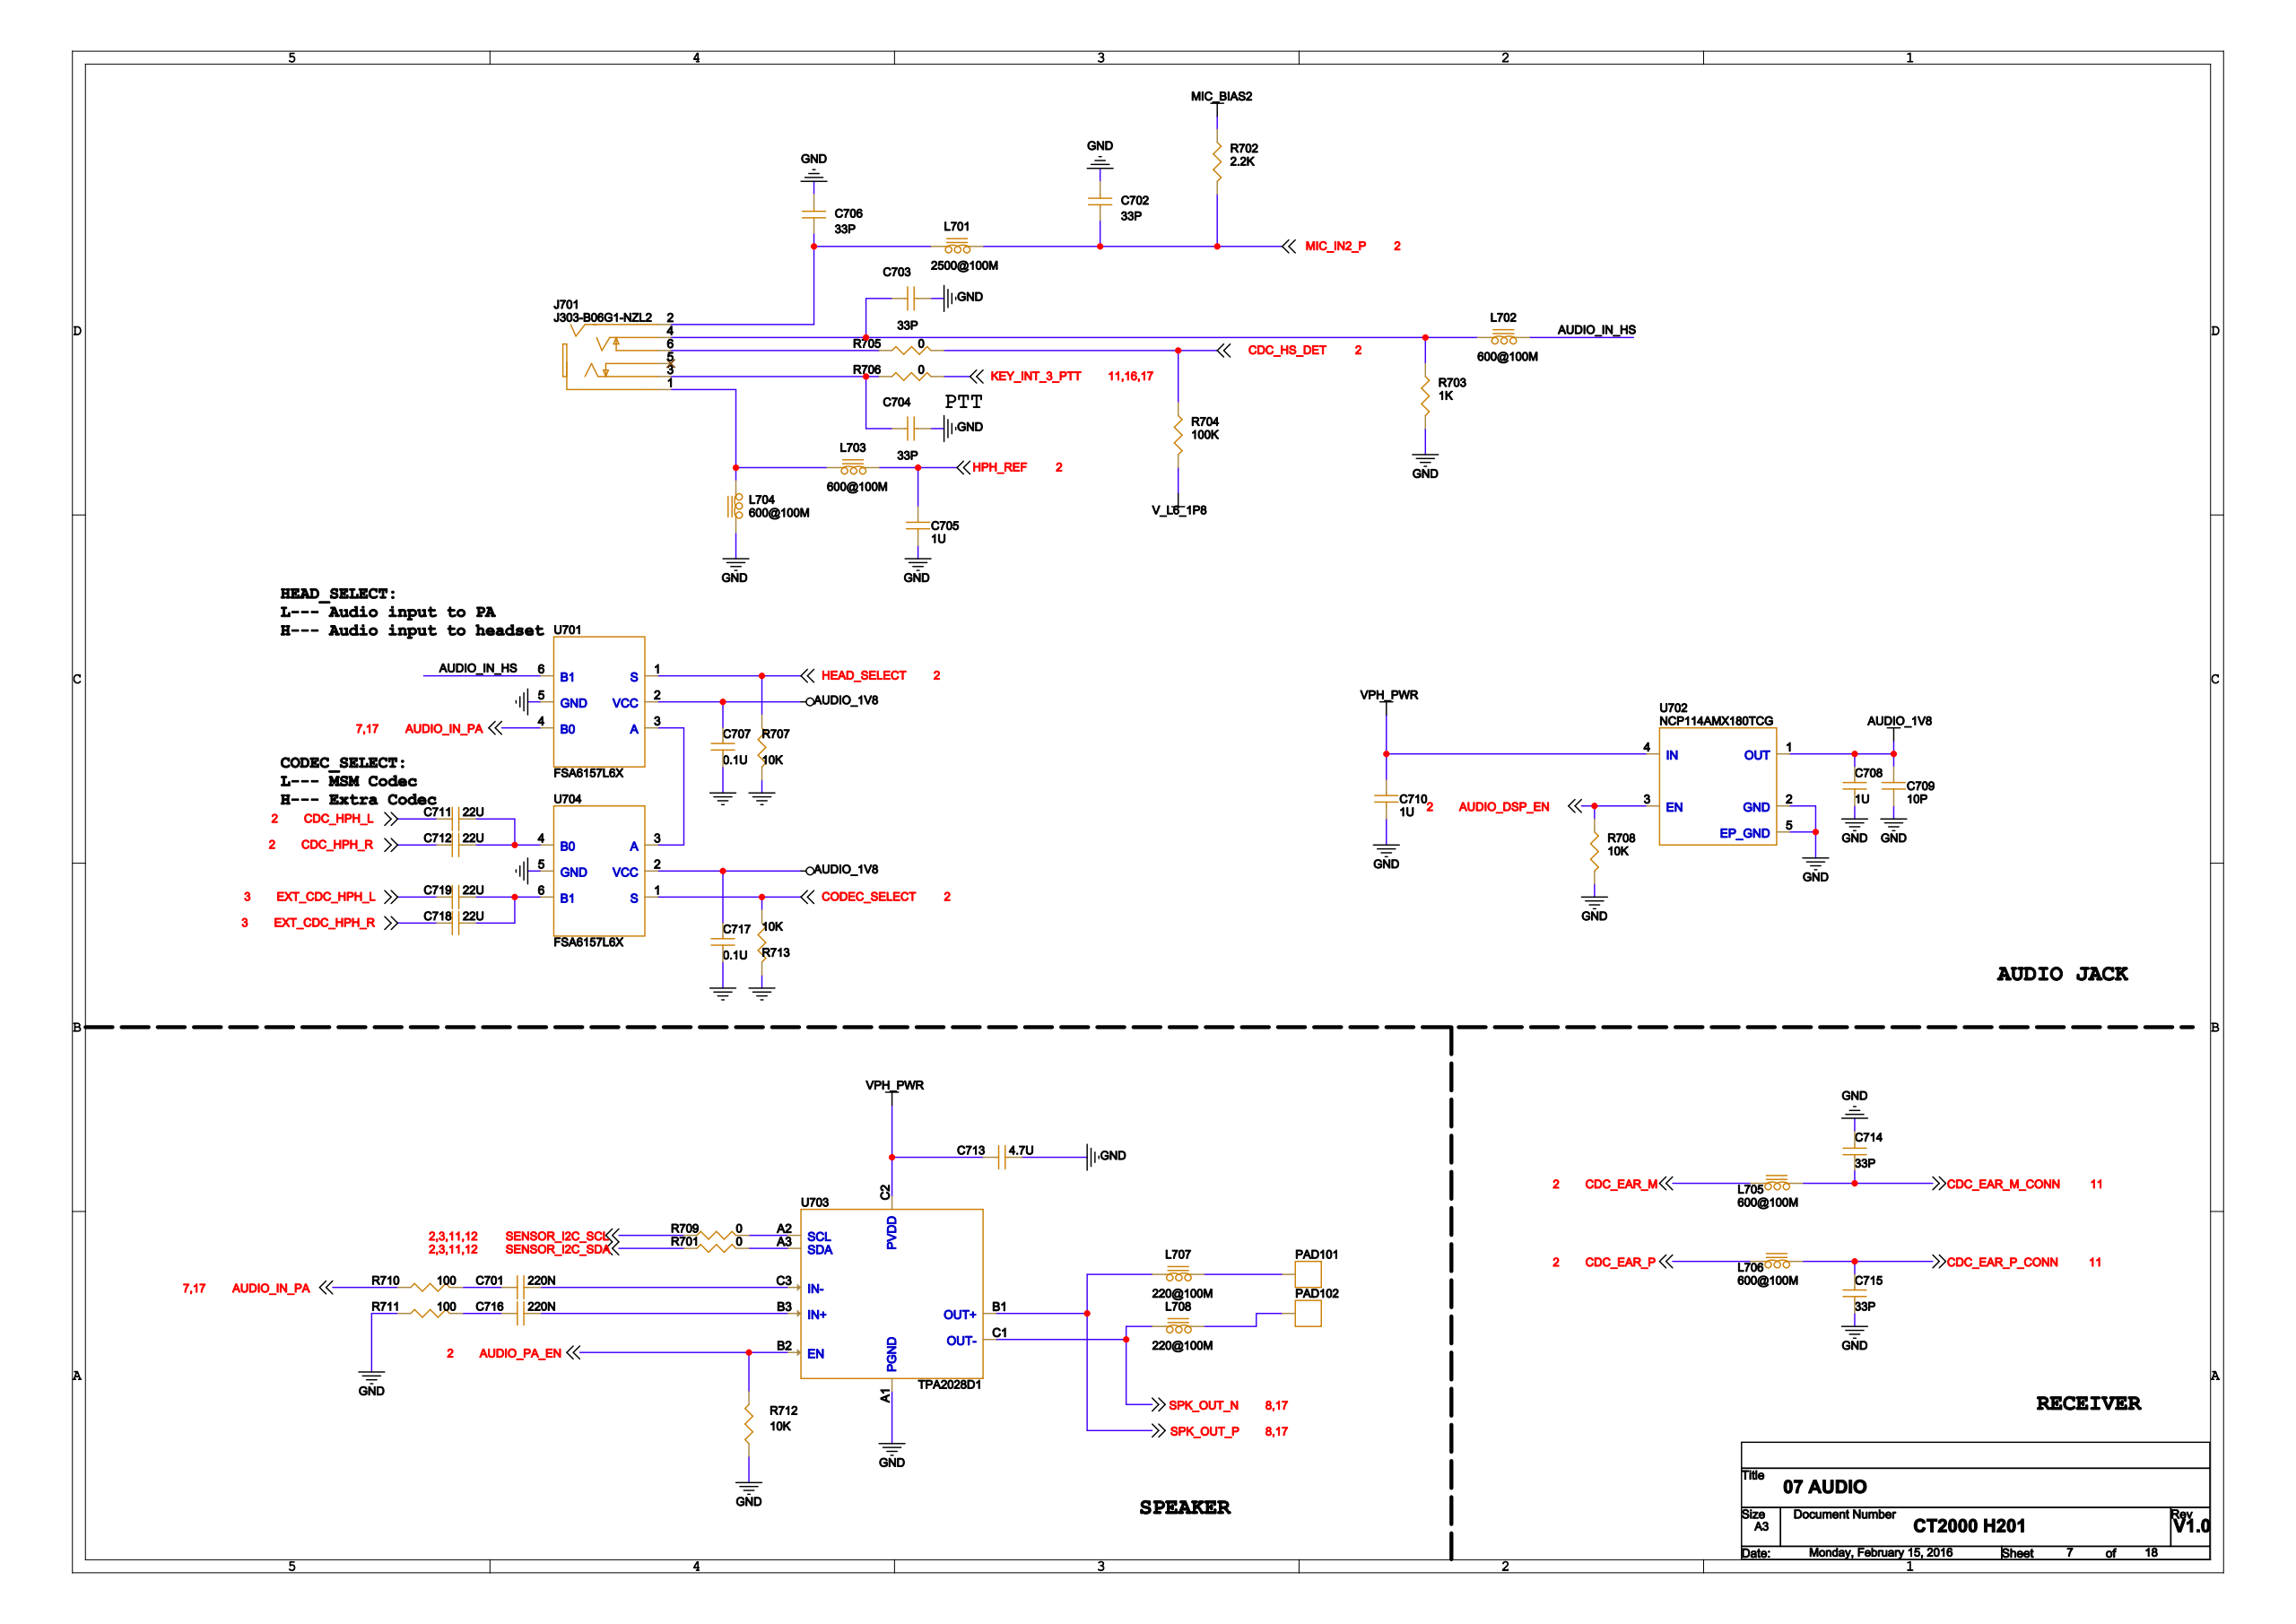Circuit board | Cadence Allegro | 573 parts | 376 nets | one sheet of the schematic
Parts on this sheet (reference | value | footprint):
C701 | 220N | C0402
C702 | 33P | C0402
C703 | 33P | C0402
C704 | 33P | C0402
C705 | 1U | C0402
C706 | 33P | C0402
C707 | 0.1U | C0402
C708 | 1U | C0402
C709 | 10P | C0402
C710 | 1U | C0402
C711 | 22U | C0805
C712 | 22U | C0805
C713 | 4.7U | C0402
C714 | 33P | C0402
C715 | 33P | C0402
C716 | 220N | C0402
C717 | 0.1U | C0402
C718 | 22U | C0805
C719 | 22U | C0805
J701 | J303-B06G1-NZL2 | JACK_J303-B06G1-NZL2
L701 | 2500@100M | L0603
L702 | 600@100M | L0402
L703 | 600@100M | L0402
L704 | 600@100M | L0402
L705 | 600@100M | L0402
L706 | 600@100M | L0402
L707 | 220@100M | L0603
L708 | 220@100M | L0603
PAD101 | PAD_R1P2X2P2 | PAD_R1P2X2P2
PAD102 | PAD_R1P2X2P2 | PAD_R1P2X2P2
R701 | 0 | R0402
R702 | 2.2K | R0402
R703 | 1K | R0402
R704 | 100K | R0402
R705 | 0 | R0402
R706 | 0 | R0402
R707 | 10K | R0402
R708 | 10K | R0402
R709 | 0 | R0402
R710 | 100 | R0402
R711 | 100 | R0402
R712 | 10K | R0402
R713 | 10K | R0402
U701 | FSA6157L6X | FSA6157L6X
U702 | NCP114AMX180TCG | UDFN4_1X1X0P7_0P65
U703 | TPA2028D1 | TPA2028D1
U704 | FSA6157L6X | FSA6157L6X
Nets of these parts (net: part-pin ...):
GND: C702-2 C703-2 C704-2 C705-2 C706-2 C707-2 C708-2 C709-2 C710-2 C713-2 C714-2 C715-2 C717-2 L704-1 R703-2 R707-2 R708-2 R711-1 R712-2 R713-1 U701-5 U702-2 U702-5 U703-A1 U704-5
N51952782: L707-2 PAD101-1
N51952794: L708-2 PAD102-1
EXT_CDC_HPH_L: C719-1
EXT_CDC_HPH_R: C718-1
KEY_INT_3_PTT: R706-2
CDC_EAR_P_CONN: C715-1 L706-2
CDC_EAR_M_CONN: C714-1 L705-2
SENSOR_I2C_SDA: R701-1
VPH_PWR: C710-1 C713-1 U702-4 U703-C2
SENSOR_I2C_SCL: R709-1
N52655103: J701-1 L703-1 L704-2
N52654966: C706-1 J701-2 L701-1
N52654932: C704-1 J701-3 R706-1
N52655055: C703-1 J701-4 L702-1 R703-1
N52654939: J701-6 R705-1
AUDIO_DSP_EN: R708-1 U702-3
AUDIO_1V8: C707-1 C708-1 C709-1 C717-1 U701-2 U702-1 U704-2
AUDIO_PA_EN: R712-1 U703-B2
CDC_EAR_M: L705-1
CDC_EAR_P: L706-1
CDC_HPH_L: C711-1
CDC_HPH_R: C712-1
CDC_HS_DET: R704-1 R705-2
HEAD_SELECT: R707-1 U701-1
HPH_REF: C705-1 L703-2
MIC_BIAS2: R702-1
MIC_IN2_P: C702-1 L701-2 R702-2
CODEC_SELECT: R713-2 U704-1
V_L6_1P8: R704-2
N52754136: C718-2 C719-2 U704-6
N52751966: C711-2 C712-2 U704-4
N51951687: C701-1 R710-2
N51938225: C701-2 U703-C3
N51951755: C716-1 R711-2
N51938227: C716-2 U703-B3
SPK_OUT_N: L708-1 U703-C1
SPK_OUT_P: L707-1 U703-B1
AUDIO_IN_HS: L702-2 U701-6
N51948767: R701-2 U703-A3
N51948732: R709-2 U703-A2
AUDIO_IN_PA: R710-1 U701-4
N52752847: U701-3 U704-3